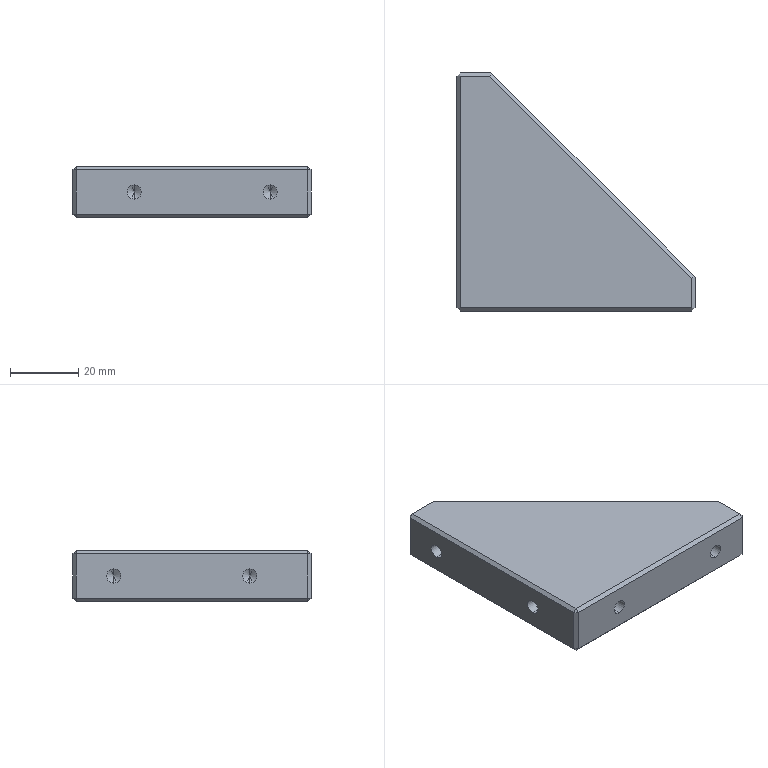Part | STEP file | BPSP-11-006Reinforcing Rib_Default | 1 solid | 42 faces | box 70 x 70 x 15 mm | volume 45416 mm3 | plane 26 | cylinder 8 | cone 8 | commonest cylinder face diameters 4.2 x8